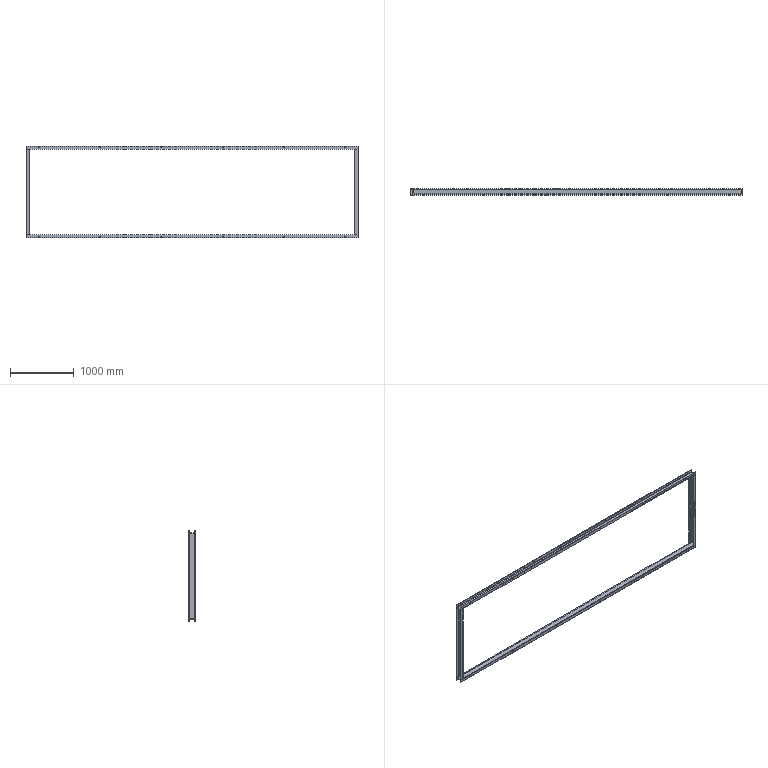Part | STEP file | SW-101-Base1_default<by machining> | 4 solids | 132 faces | box 5206 x 100 x 1440 mm | volume 16389310 mm3 | cylinder 92 | plane 40 | commonest cylinder face diameters 20 x52 18 x24 8.5 x8 17 x8